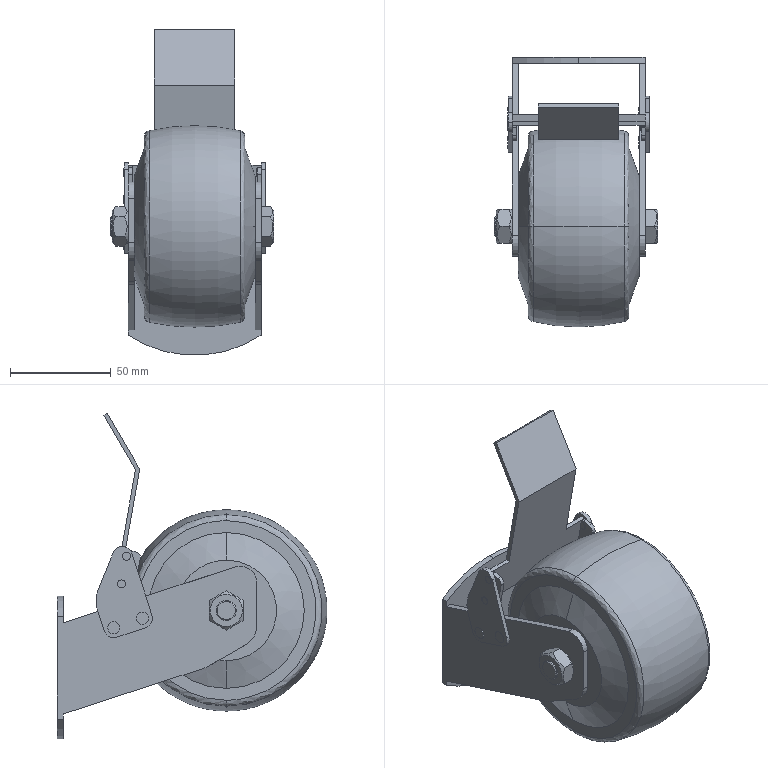Part | STEP file | _CEL21-100-P-001 | 1 solid | 166 faces | box 81.4 x 134 x 162 mm | volume 463368 mm3 | plane 81 | cylinder 67 | cone 12 | spline 4 | torus 2 | commonest cylinder face diameters 6 x26 4 x20 10 x10 118.9 x3 16 x2 20 x2